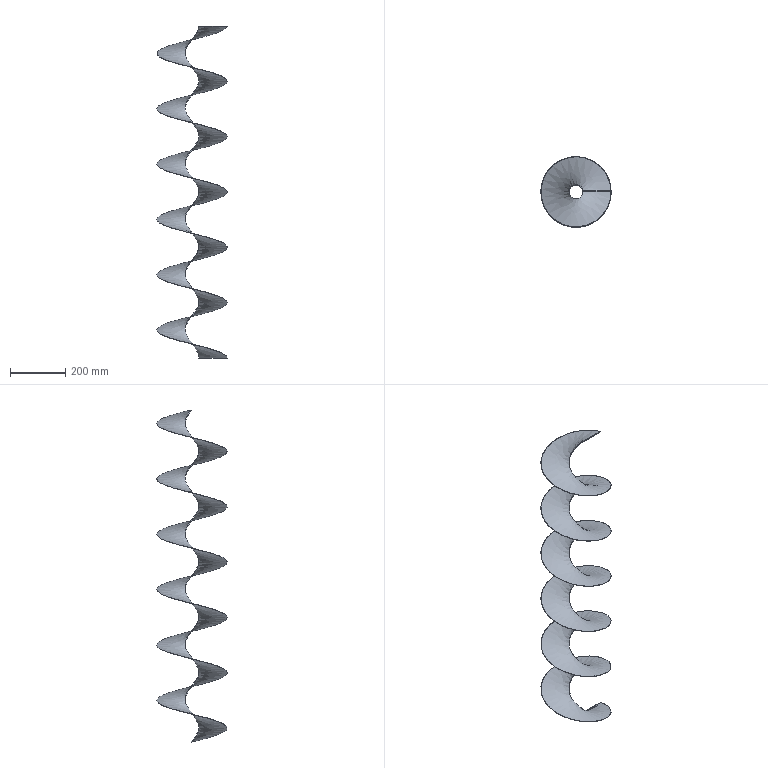Part | SolidWorks | features BaseBody 1 | 1 solid | 6 faces | box 253.758 x 253.748 x 1200 mm | volume 425695 mm3 | spline 4 | plane 2